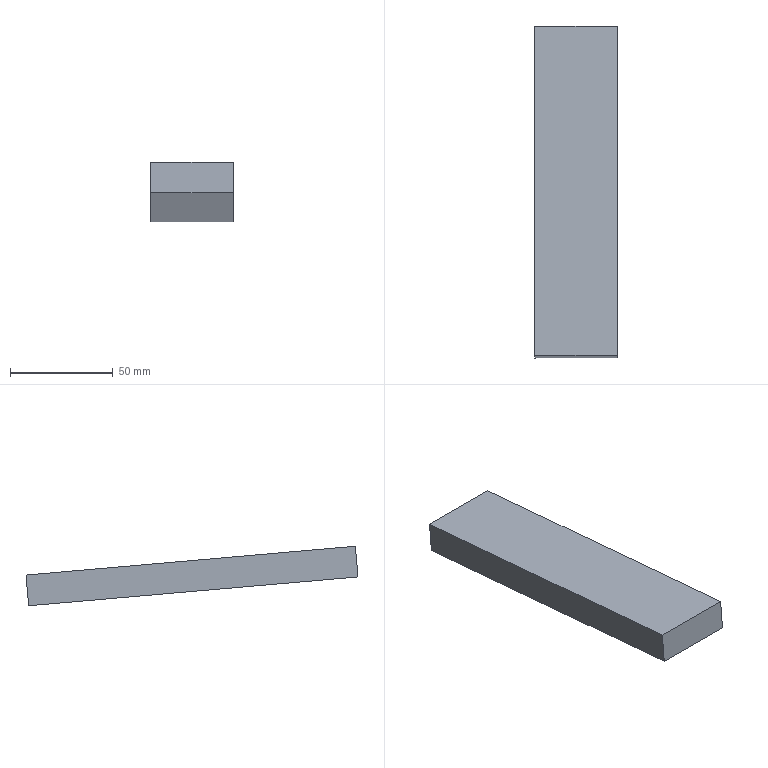Part | NX | features solid 2 | 1 solid | 6 faces | box 40 x 161.307 x 28.941 mm | volume 96367 mm3 | plane 6
STEP:
#1=CARTESIAN_POINT('',(-607.,658.693,124.386));
#2=VERTEX_POINT('',#1);
#3=CARTESIAN_POINT('',(-607.,660.,139.329));
#4=VERTEX_POINT('',#3);
#5=CARTESIAN_POINT('',(-607.,658.693,124.386));
#6=DIRECTION('',(0.,0.08716,0.9962));
#7=VECTOR('',#6,1000.);
#8=LINE('',#5,#7);
#9=EDGE_CURVE('',#2,#4,#8,.T.);
#10=ORIENTED_EDGE('',*,*,#9,.F.);
#11=CARTESIAN_POINT('',(-567.,658.693,124.386));
#12=VERTEX_POINT('',#11);
#13=CARTESIAN_POINT('',(-610.,658.693,124.386));
#14=DIRECTION('',(1.,0.,0.));
#15=VECTOR('',#14,1000.);
#16=LINE('',#13,#15);
#17=EDGE_CURVE('',#2,#12,#16,.T.);
#18=ORIENTED_EDGE('',*,*,#17,.T.);
#19=CARTESIAN_POINT('',(-567.,660.,139.329));
#20=VERTEX_POINT('',#19);
#21=CARTESIAN_POINT('',(-567.,658.693,124.386));
#22=DIRECTION('',(0.,0.08716,0.9962));
#23=VECTOR('',#22,1000.);
#24=LINE('',#21,#23);
#25=EDGE_CURVE('',#12,#20,#24,.T.);
#26=ORIENTED_EDGE('',*,*,#25,.T.);
#27=CARTESIAN_POINT('',(-610.,660.,139.329));
#28=DIRECTION('',(1.,0.,0.));
#29=VECTOR('',#28,1000.);
#30=LINE('',#27,#29);
#31=EDGE_CURVE('',#4,#20,#30,.T.);
#32=ORIENTED_EDGE('',*,*,#31,.F.);
#33=EDGE_LOOP('',(#10,#18,#26,#32));
#34=FACE_BOUND('',#33,.T.);
#35=CARTESIAN_POINT('',(-610.,658.693,124.386));
#36=DIRECTION('',(0.,0.9962,-0.08716));
#37=DIRECTION('',(0.,-0.08716,-0.9962));
#38=AXIS2_PLACEMENT_3D('',#35,#36,#37);
#39=PLANE('',#38);
#40=ADVANCED_FACE('',(#34),#39,.F.);
#41=CARTESIAN_POINT('',(-607.,820.,125.33));
#42=VERTEX_POINT('',#41);
#43=CARTESIAN_POINT('',(-567.,820.,125.33));
#44=VERTEX_POINT('',#43);
#45=CARTESIAN_POINT('',(-610.,820.,125.33));
#46=DIRECTION('',(1.,0.,0.));
#47=VECTOR('',#46,1000.);
#48=LINE('',#45,#47);
#49=EDGE_CURVE('',#42,#44,#48,.T.);
#50=ORIENTED_EDGE('',*,*,#49,.T.);
#51=CARTESIAN_POINT('',(-567.,818.693,110.387));
#52=VERTEX_POINT('',#51);
#53=CARTESIAN_POINT('',(-567.,818.693,110.387));
#54=DIRECTION('',(0.,0.08716,0.9962));
#55=VECTOR('',#54,1000.);
#56=LINE('',#53,#55);
#57=EDGE_CURVE('',#52,#44,#56,.T.);
#58=ORIENTED_EDGE('',*,*,#57,.F.);
#59=CARTESIAN_POINT('',(-607.,818.693,110.387));
#60=VERTEX_POINT('',#59);
#61=CARTESIAN_POINT('',(-610.,818.693,110.387));
#62=DIRECTION('',(1.,0.,0.));
#63=VECTOR('',#62,1000.);
#64=LINE('',#61,#63);
#65=EDGE_CURVE('',#60,#52,#64,.T.);
#66=ORIENTED_EDGE('',*,*,#65,.F.);
#67=CARTESIAN_POINT('',(-607.,818.693,110.387));
#68=DIRECTION('',(0.,0.08716,0.9962));
#69=VECTOR('',#68,1000.);
#70=LINE('',#67,#69);
#71=EDGE_CURVE('',#60,#42,#70,.T.);
#72=ORIENTED_EDGE('',*,*,#71,.T.);
#73=EDGE_LOOP('',(#50,#58,#66,#72));
#74=FACE_BOUND('',#73,.T.);
#75=CARTESIAN_POINT('',(-610.,818.693,110.387));
#76=DIRECTION('',(0.,0.9962,-0.08716));
#77=DIRECTION('',(0.,-0.08716,-0.9962));
#78=AXIS2_PLACEMENT_3D('',#75,#76,#77);
#79=PLANE('',#78);
#80=ADVANCED_FACE('',(#74),#79,.T.);
#81=ORIENTED_EDGE('',*,*,#65,.T.);
#82=CARTESIAN_POINT('',(-567.,818.693,110.387));
#83=DIRECTION('',(0.,-0.9962,0.08716));
#84=VECTOR('',#83,1000.);
#85=LINE('',#82,#84);
#86=EDGE_CURVE('',#52,#12,#85,.T.);
#87=ORIENTED_EDGE('',*,*,#86,.T.);
#88=ORIENTED_EDGE('',*,*,#17,.F.);
#89=CARTESIAN_POINT('',(-607.,658.693,124.386));
#90=DIRECTION('',(0.,0.9962,-0.08716));
#91=VECTOR('',#90,1000.);
#92=LINE('',#89,#91);
#93=EDGE_CURVE('',#2,#60,#92,.T.);
#94=ORIENTED_EDGE('',*,*,#93,.T.);
#95=EDGE_LOOP('',(#81,#87,#88,#94));
#96=FACE_BOUND('',#95,.T.);
#97=CARTESIAN_POINT('',(-565.,818.693,110.387));
#98=DIRECTION('',(0.,-0.08716,-0.9962));
#99=DIRECTION('',(0.,-0.9962,0.08716));
#100=AXIS2_PLACEMENT_3D('',#97,#98,#99);
#101=PLANE('',#100);
#102=ADVANCED_FACE('',(#96),#101,.T.);
#103=CARTESIAN_POINT('',(-607.,660.,139.329));
#104=DIRECTION('',(0.,0.9962,-0.08716));
#105=VECTOR('',#104,1000.);
#106=LINE('',#103,#105);
#107=EDGE_CURVE('',#4,#42,#106,.T.);
#108=ORIENTED_EDGE('',*,*,#107,.F.);
#109=ORIENTED_EDGE('',*,*,#31,.T.);
#110=CARTESIAN_POINT('',(-567.,820.,125.33));
#111=DIRECTION('',(0.,-0.9962,0.08716));
#112=VECTOR('',#111,1000.);
#113=LINE('',#110,#112);
#114=EDGE_CURVE('',#44,#20,#113,.T.);
#115=ORIENTED_EDGE('',*,*,#114,.F.);
#116=ORIENTED_EDGE('',*,*,#49,.F.);
#117=EDGE_LOOP('',(#108,#109,#115,#116));
#118=FACE_BOUND('',#117,.T.);
#119=CARTESIAN_POINT('',(-565.,820.,125.33));
#120=DIRECTION('',(0.,-0.08716,-0.9962));
#121=DIRECTION('',(0.,-0.9962,0.08716));
#122=AXIS2_PLACEMENT_3D('',#119,#120,#121);
#123=PLANE('',#122);
#124=ADVANCED_FACE('',(#118),#123,.F.);
#125=ORIENTED_EDGE('',*,*,#114,.T.);
#126=ORIENTED_EDGE('',*,*,#25,.F.);
#127=ORIENTED_EDGE('',*,*,#86,.F.);
#128=ORIENTED_EDGE('',*,*,#57,.T.);
#129=EDGE_LOOP('',(#125,#126,#127,#128));
#130=FACE_BOUND('',#129,.T.);
#131=CARTESIAN_POINT('',(-567.,818.693,110.387));
#132=DIRECTION('',(1.,0.,0.));
#133=DIRECTION('',(0.,-1.,0.));
#134=AXIS2_PLACEMENT_3D('',#131,#132,#133);
#135=PLANE('',#134);
#136=ADVANCED_FACE('',(#130),#135,.T.);
#137=ORIENTED_EDGE('',*,*,#107,.T.);
#138=ORIENTED_EDGE('',*,*,#71,.F.);
#139=ORIENTED_EDGE('',*,*,#93,.F.);
#140=ORIENTED_EDGE('',*,*,#9,.T.);
#141=EDGE_LOOP('',(#137,#138,#139,#140));
#142=FACE_BOUND('',#141,.T.);
#143=CARTESIAN_POINT('',(-607.,658.693,124.386));
#144=DIRECTION('',(-1.,0.,0.));
#145=DIRECTION('',(0.,1.,0.));
#146=AXIS2_PLACEMENT_3D('',#143,#144,#145);
#147=PLANE('',#146);
#148=ADVANCED_FACE('',(#142),#147,.T.);
#149=CLOSED_SHELL('',(#40,#80,#102,#124,#136,#148));
#150=MANIFOLD_SOLID_BREP('',#149);
#151=(LENGTH_UNIT()NAMED_UNIT(*)SI_UNIT(.MILLI.,.METRE.));
#152=UNCERTAINTY_MEASURE_WITH_UNIT(LENGTH_MEASURE(0.00001),#151,'','');
#153=(NAMED_UNIT(*)PLANE_ANGLE_UNIT()SI_UNIT($,.RADIAN.));
#154=(NAMED_UNIT(*)SI_UNIT($,.STERADIAN.)SOLID_ANGLE_UNIT());
#155=(GEOMETRIC_REPRESENTATION_CONTEXT(3)GLOBAL_UNCERTAINTY_ASSIGNED_CONTEXT((#152))GLOBAL_UNIT_ASSIGNED_CONTEXT((#151,#153,#154))REPRESENTATION_CONTEXT('',''));
#156=ADVANCED_BREP_SHAPE_REPRESENTATION('',(#150),#155);